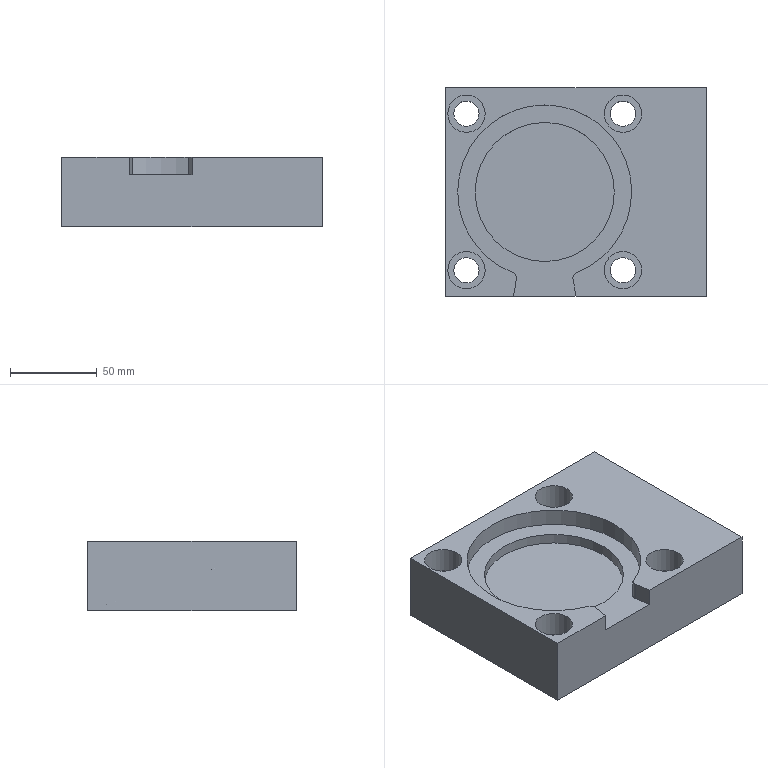NC program | NX | posted with a generic post | part box 150 x 120 x 40 mm
Lines 1 to 31 of 1997:
N10 G17 G21 G94 G90
(DRILLING , TOOL : D6A45)
N12 T07 M6
N14 G54
N16 G17 G0 G90 X27. Y-45. S5000 M3
N18 G43 Z30. H7
N20 G94 G81 G98 Z-1. F250. R3.
N22 X-63.
N24 Y45.
N26 X27.
N28 G80
N30 G0 X27. Y45. Z30.
N32 M5
(DRILLING_COPY , TOOL : 14.5ZT)
N34 T14 M6
N36 G54
N38 G17 G0 G90 X27. Y-45. S1200 M3
N40 G43 Z30. H14
N42 G94 G83 G98 Z-44.356 F200. Q2. R3.
N44 X-63.
N46 Y45.
N48 X27.
N50 G80
N52 G0 X27. Y45. Z30.
N54 M5